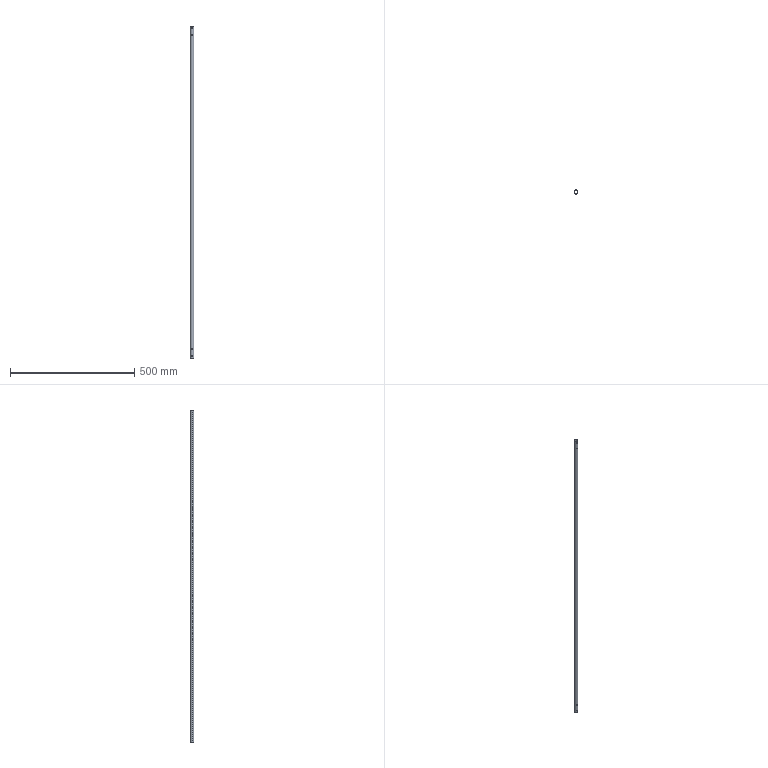Part | SolidWorks | features Extrusion 1, ICE 1 | 1 solid | 22 faces | box 14 x 14 x 1336 mm | volume 28300 mm3 | cylinder 20 | plane 2 | commonest cylinder face diameters 3.1 x16 13 x2 14 x2